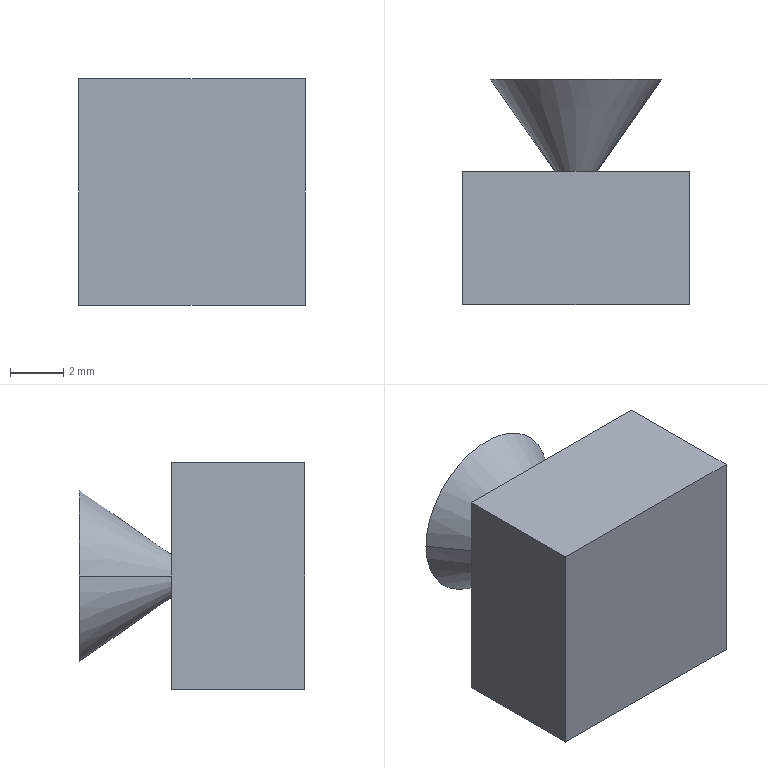Part | Creo | 1 solid | 14 faces | box 8.5 x 8.45 x 8.5 mm | volume 356.367 mm3 | plane 8 | cylinder 4 | cone 2 | commonest cylinder face diameters 6 x2 6.6 x2